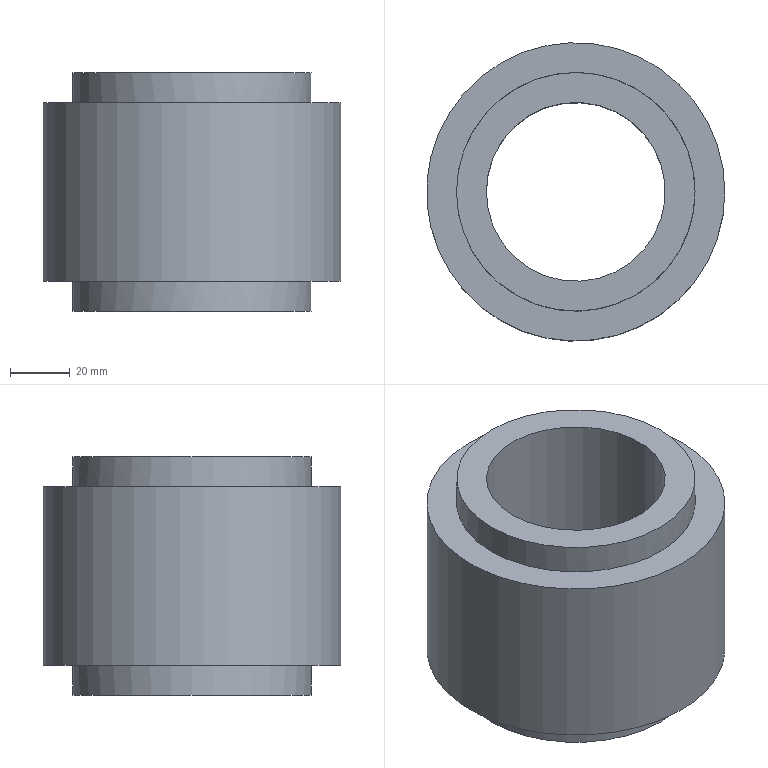Part | NX | features DATUM_CSYS 3, EXTRUDE 2, SKETCH 2, HOLE PACKAGE 1, SIMPLE HOLE 1 | 1 solid | 8 faces | box 100 x 100 x 80 mm | volume 345575 mm3 | cylinder 4 | plane 4 | commonest cylinder face diameters 80 x2 60 x1 100 x1
STEP:
#1=CARTESIAN_POINT('',(40.,0.,40.));
#2=VERTEX_POINT('',#1);
#3=CARTESIAN_POINT('',(0.,0.,40.));
#4=DIRECTION('',(0.,0.,-1.));
#5=DIRECTION('',(1.,0.,0.));
#6=AXIS2_PLACEMENT_3D('',#3,#4,#5);
#7=CIRCLE('',#6,40.);
#8=EDGE_CURVE('',#2,#2,#7,.T.);
#9=ORIENTED_EDGE('',*,*,#8,.T.);
#10=EDGE_LOOP('',(#9));
#11=FACE_BOUND('',#10,.T.);
#12=CARTESIAN_POINT('',(-40.,0.,30.));
#13=VERTEX_POINT('',#12);
#14=CARTESIAN_POINT('',(0.,0.,30.));
#15=DIRECTION('',(0.,0.,-1.));
#16=DIRECTION('',(-1.,0.,0.));
#17=AXIS2_PLACEMENT_3D('',#14,#15,#16);
#18=CIRCLE('',#17,40.);
#19=EDGE_CURVE('',#13,#13,#18,.F.);
#20=ORIENTED_EDGE('',*,*,#19,.T.);
#21=EDGE_LOOP('',(#20));
#22=FACE_BOUND('',#21,.T.);
#23=CARTESIAN_POINT('',(0.,0.,40.));
#24=DIRECTION('',(0.,0.,-1.));
#25=DIRECTION('',(-1.,0.,0.));
#26=AXIS2_PLACEMENT_3D('',#23,#24,#25);
#27=CYLINDRICAL_SURFACE('',#26,40.);
#28=ADVANCED_FACE('',(#11,#22),#27,.T.);
#29=CARTESIAN_POINT('',(-30.,0.,40.));
#30=VERTEX_POINT('',#29);
#31=CARTESIAN_POINT('',(0.,0.,40.));
#32=DIRECTION('',(0.,0.,-1.));
#33=DIRECTION('',(-1.,0.,0.));
#34=AXIS2_PLACEMENT_3D('',#31,#32,#33);
#35=CIRCLE('',#34,30.);
#36=EDGE_CURVE('',#30,#30,#35,.T.);
#37=ORIENTED_EDGE('',*,*,#36,.T.);
#38=EDGE_LOOP('',(#37));
#39=FACE_BOUND('',#38,.T.);
#40=ORIENTED_EDGE('',*,*,#8,.F.);
#41=EDGE_LOOP('',(#40));
#42=FACE_BOUND('',#41,.T.);
#43=CARTESIAN_POINT('',(0.,0.,40.));
#44=DIRECTION('',(0.,0.,-1.));
#45=DIRECTION('',(-1.,0.,0.));
#46=AXIS2_PLACEMENT_3D('',#43,#44,#45);
#47=PLANE('',#46);
#48=ADVANCED_FACE('',(#39,#42),#47,.F.);
#49=CARTESIAN_POINT('',(50.,0.,30.));
#50=VERTEX_POINT('',#49);
#51=CARTESIAN_POINT('',(0.,0.,30.));
#52=DIRECTION('',(0.,0.,-1.));
#53=DIRECTION('',(1.,0.,0.));
#54=AXIS2_PLACEMENT_3D('',#51,#52,#53);
#55=CIRCLE('',#54,50.);
#56=EDGE_CURVE('',#50,#50,#55,.T.);
#57=ORIENTED_EDGE('',*,*,#56,.T.);
#58=EDGE_LOOP('',(#57));
#59=FACE_BOUND('',#58,.T.);
#60=CARTESIAN_POINT('',(50.,0.,-30.));
#61=VERTEX_POINT('',#60);
#62=CARTESIAN_POINT('',(0.,0.,-30.));
#63=DIRECTION('',(0.,0.,-1.));
#64=DIRECTION('',(1.,0.,0.));
#65=AXIS2_PLACEMENT_3D('',#62,#63,#64);
#66=CIRCLE('',#65,50.);
#67=EDGE_CURVE('',#61,#61,#66,.T.);
#68=ORIENTED_EDGE('',*,*,#67,.F.);
#69=EDGE_LOOP('',(#68));
#70=FACE_BOUND('',#69,.T.);
#71=CARTESIAN_POINT('',(0.,0.,30.));
#72=DIRECTION('',(0.,0.,-1.));
#73=DIRECTION('',(-1.,0.,0.));
#74=AXIS2_PLACEMENT_3D('',#71,#72,#73);
#75=CYLINDRICAL_SURFACE('',#74,50.);
#76=ADVANCED_FACE('',(#59,#70),#75,.T.);
#77=ORIENTED_EDGE('',*,*,#19,.F.);
#78=EDGE_LOOP('',(#77));
#79=FACE_BOUND('',#78,.T.);
#80=ORIENTED_EDGE('',*,*,#56,.F.);
#81=EDGE_LOOP('',(#80));
#82=FACE_BOUND('',#81,.T.);
#83=CARTESIAN_POINT('',(0.,0.,30.));
#84=DIRECTION('',(0.,0.,-1.));
#85=DIRECTION('',(-1.,0.,0.));
#86=AXIS2_PLACEMENT_3D('',#83,#84,#85);
#87=PLANE('',#86);
#88=ADVANCED_FACE('',(#79,#82),#87,.F.);
#89=CARTESIAN_POINT('',(-40.,0.,-30.));
#90=VERTEX_POINT('',#89);
#91=CARTESIAN_POINT('',(0.,0.,-30.));
#92=DIRECTION('',(0.,0.,-1.));
#93=DIRECTION('',(-1.,0.,0.));
#94=AXIS2_PLACEMENT_3D('',#91,#92,#93);
#95=CIRCLE('',#94,40.);
#96=EDGE_CURVE('',#90,#90,#95,.F.);
#97=ORIENTED_EDGE('',*,*,#96,.T.);
#98=EDGE_LOOP('',(#97));
#99=FACE_BOUND('',#98,.T.);
#100=ORIENTED_EDGE('',*,*,#67,.T.);
#101=EDGE_LOOP('',(#100));
#102=FACE_BOUND('',#101,.T.);
#103=CARTESIAN_POINT('',(0.,0.,-30.));
#104=DIRECTION('',(0.,0.,-1.));
#105=DIRECTION('',(-1.,0.,0.));
#106=AXIS2_PLACEMENT_3D('',#103,#104,#105);
#107=PLANE('',#106);
#108=ADVANCED_FACE('',(#99,#102),#107,.T.);
#109=CARTESIAN_POINT('',(-30.,0.,-40.));
#110=VERTEX_POINT('',#109);
#111=CARTESIAN_POINT('',(0.,0.,-40.));
#112=DIRECTION('',(0.,0.,-1.));
#113=DIRECTION('',(-1.,0.,0.));
#114=AXIS2_PLACEMENT_3D('',#111,#112,#113);
#115=CIRCLE('',#114,30.);
#116=EDGE_CURVE('',#110,#110,#115,.T.);
#117=ORIENTED_EDGE('',*,*,#116,.F.);
#118=EDGE_LOOP('',(#117));
#119=FACE_BOUND('',#118,.T.);
#120=CARTESIAN_POINT('',(40.,0.,-40.));
#121=VERTEX_POINT('',#120);
#122=CARTESIAN_POINT('',(0.,0.,-40.));
#123=DIRECTION('',(0.,0.,-1.));
#124=DIRECTION('',(1.,0.,0.));
#125=AXIS2_PLACEMENT_3D('',#122,#123,#124);
#126=CIRCLE('',#125,40.);
#127=EDGE_CURVE('',#121,#121,#126,.T.);
#128=ORIENTED_EDGE('',*,*,#127,.T.);
#129=EDGE_LOOP('',(#128));
#130=FACE_BOUND('',#129,.T.);
#131=CARTESIAN_POINT('',(0.,0.,-40.));
#132=DIRECTION('',(0.,0.,-1.));
#133=DIRECTION('',(-1.,0.,0.));
#134=AXIS2_PLACEMENT_3D('',#131,#132,#133);
#135=PLANE('',#134);
#136=ADVANCED_FACE('',(#119,#130),#135,.T.);
#137=ORIENTED_EDGE('',*,*,#96,.F.);
#138=EDGE_LOOP('',(#137));
#139=FACE_BOUND('',#138,.T.);
#140=ORIENTED_EDGE('',*,*,#127,.F.);
#141=EDGE_LOOP('',(#140));
#142=FACE_BOUND('',#141,.T.);
#143=CARTESIAN_POINT('',(0.,0.,40.));
#144=DIRECTION('',(0.,0.,-1.));
#145=DIRECTION('',(-1.,0.,0.));
#146=AXIS2_PLACEMENT_3D('',#143,#144,#145);
#147=CYLINDRICAL_SURFACE('',#146,40.);
#148=ADVANCED_FACE('',(#139,#142),#147,.T.);
#149=ORIENTED_EDGE('',*,*,#116,.T.);
#150=EDGE_LOOP('',(#149));
#151=FACE_BOUND('',#150,.T.);
#152=ORIENTED_EDGE('',*,*,#36,.F.);
#153=EDGE_LOOP('',(#152));
#154=FACE_BOUND('',#153,.T.);
#155=CARTESIAN_POINT('',(0.,0.,40.));
#156=DIRECTION('',(0.,0.,-1.));
#157=DIRECTION('',(-1.,0.,0.));
#158=AXIS2_PLACEMENT_3D('',#155,#156,#157);
#159=CYLINDRICAL_SURFACE('',#158,30.);
#160=ADVANCED_FACE('',(#151,#154),#159,.F.);
#161=CLOSED_SHELL('',(#28,#48,#76,#88,#108,#136,#148,#160));
#162=MANIFOLD_SOLID_BREP('',#161);
#163=(LENGTH_UNIT()NAMED_UNIT(*)SI_UNIT(.MILLI.,.METRE.));
#164=UNCERTAINTY_MEASURE_WITH_UNIT(LENGTH_MEASURE(0.00001),#163,'','');
#165=(NAMED_UNIT(*)PLANE_ANGLE_UNIT()SI_UNIT($,.RADIAN.));
#166=(NAMED_UNIT(*)SI_UNIT($,.STERADIAN.)SOLID_ANGLE_UNIT());
#167=(GEOMETRIC_REPRESENTATION_CONTEXT(3)GLOBAL_UNCERTAINTY_ASSIGNED_CONTEXT((#164))GLOBAL_UNIT_ASSIGNED_CONTEXT((#163,#165,#166))REPRESENTATION_CONTEXT('',''));
#168=ADVANCED_BREP_SHAPE_REPRESENTATION('',(#162),#167);